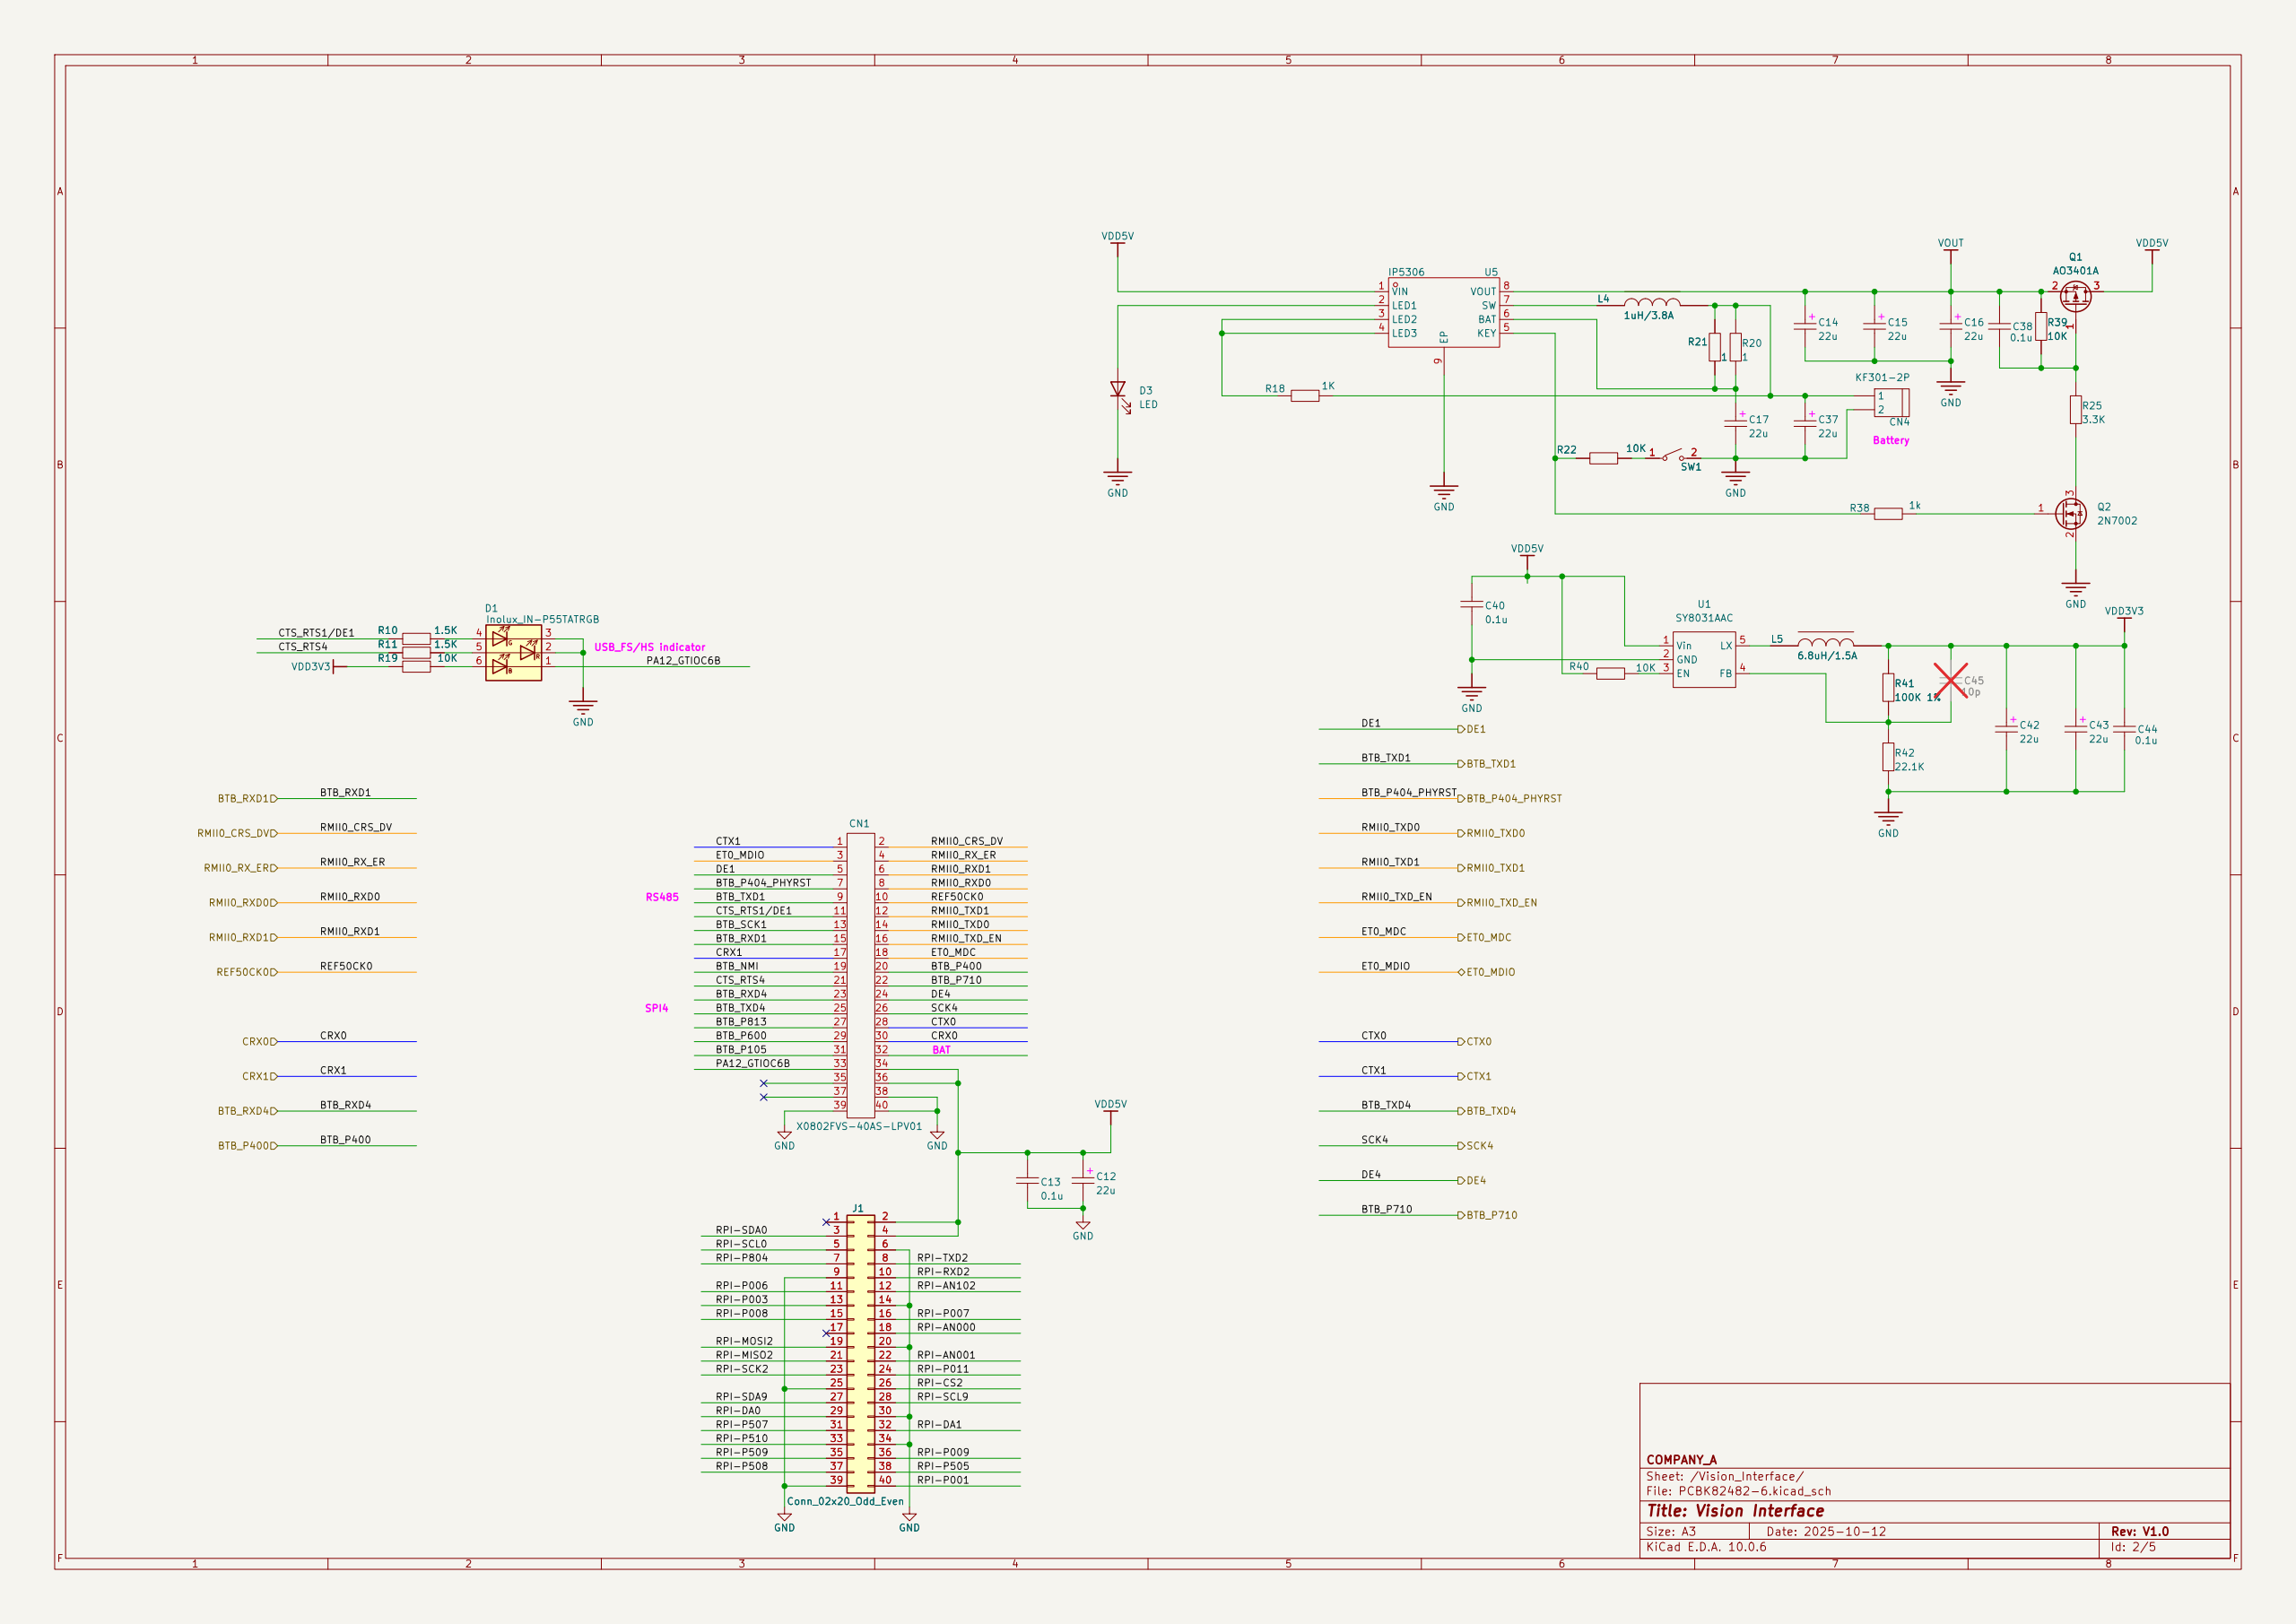Circuit board | KiCad | 154 parts | 201 nets | one sheet of the schematic
Parts on this sheet (reference | value | footprint):
C12 | 22u | Library:C1206
C13 | 0.1u | Library:C0603
C14
C15
C16
C17
C37 | 22u | Library:C1206
C38 | 0.1u | Library:C0603
C40 | 0.1u | Library:C0603
C42 | 22u | Library:C1206
C43 | 22u | Library:C1206
C44 | 0.1u | Library:C0603
C45
CN1 | X0802FVS-40AS-LPV01 | Library:CONN-SMD_40P-P0.80-Mu
CN4 | KF301-2P | Library:HEAD2L-0.8
D1 | Inolux_IN-P55TATRGB | LED_SMD:LED_Inolux_IN-P55TATRGB_PLCC6_5.0x5.5mm_P1.8mm
D3 | LED | LED_SMD:LED_0603_1608Metric
J1 | Conn_02x20_Odd_Even | Connector_PinHeader_2.54mm:PinHeader_2x20_P2.54mm_Vertical
L4 | 1uH/3.8A | Library:PL0505
L5 | 6.8uH/1.5A | Library:PL0505
Q1 | AO3401A | Package_TO_SOT_SMD:SOT-23
Q2 | 2N7002 | Package_TO_SOT_SMD:SOT-23
R10 | 1.5K | Library:R0603
R11 | 1.5K | Library:R0603
R18 | 1K | Resistor_SMD:R_0402_1005Metric_Pad0.72x0.64mm_HandSolder
R19 | 10K | Library:R0603
R20 | 1 | Library:R0603
R21 | 1 | Library:R0603
R22 | 10K | Library:R0603
R25 | 3.3K | Library:R0603
R38 | 1k | Library:R0603
R39 | 10K | Library:R0603
R40 | 10K | Library:R0603
R41 | 100K 1% | Library:R0603
R42 | 22.1K | Library:R0603
SW1 | TS-1088R-02026 | Library:SW-SMD_L3.9-W3.0-P4.45
U1 | SY8031AAC | Library:SOT23-5-I38-100
U5 | IP5306 | Library:ESOP-8_L4.9-W3.9-P1.27-LS6.0-BL-EP
Nets of these parts (net: part-pin ...):
/Vision_Interface/CTS_RTS1{slash}DE1: R10-2 CN1-11
/Vision_Interface/CTS_RTS4: R11-2 CN1-21
/Vision_Interface/PA12_GTIOC6B: D1-1 CN1-33
GND: C12-2 C13-1 C14-2 C15-2 C16-2 C17-2 C37-2 C40-1 C42-2 C43-2 C44-1 CN4-2 D1-2 D1-3 D3-1 Q2-2 R42-1 SW1-2 U1-2 U5-9 CN1-38 CN1-39 CN1-40 J1-6 J1-9 J1-14 J1-20 J1-25 J1-30 J1-34 J1-39
Net-(C37-Pad1): C37-1 CN4-1 L4-2 R18-1 R20-2 R21-2
Net-(D1-AB): D1-6 R19-1
Net-(D1-AG): D1-4 R10-1
Net-(D1-AR): D1-5 R11-1
Net-(D3-A): D3-2 U5-2
Net-(Q1-G): C38-1 Q1-1 R25-2 R39-1
Net-(Q2-D): Q2-3 R25-1
Net-(Q2-G): Q2-1 R38-2
Net-(R22-Pad1): R22-1 SW1-1
Net-(U1-EN): R40-1 U1-3
Net-(U1-FB): C45-1 R41-1 R42-2 U1-4
Net-(U1-LX): L5-1 U1-5
Net-(U5-BAT): C17-1 R20-1 R21-1 U5-6
Net-(U5-KEY): R22-2 R38-1 U5-5
Net-(U5-LED2): R18-2 U5-3 U5-4
Net-(U5-SW): L4-1 U5-7
VDD3V3: C42-1 C43-1 C44-2 C45-2 L5-2 R19-2 R41-2
VDD5V: C12-1 C13-2 C40-2 Q1-3 R40-2 U1-1 U5-1 CN1-34 CN1-36 J1-2 J1-4
VOUT: C14-1 C15-1 C16-1 C38-2 Q1-2 R39-2 U5-8